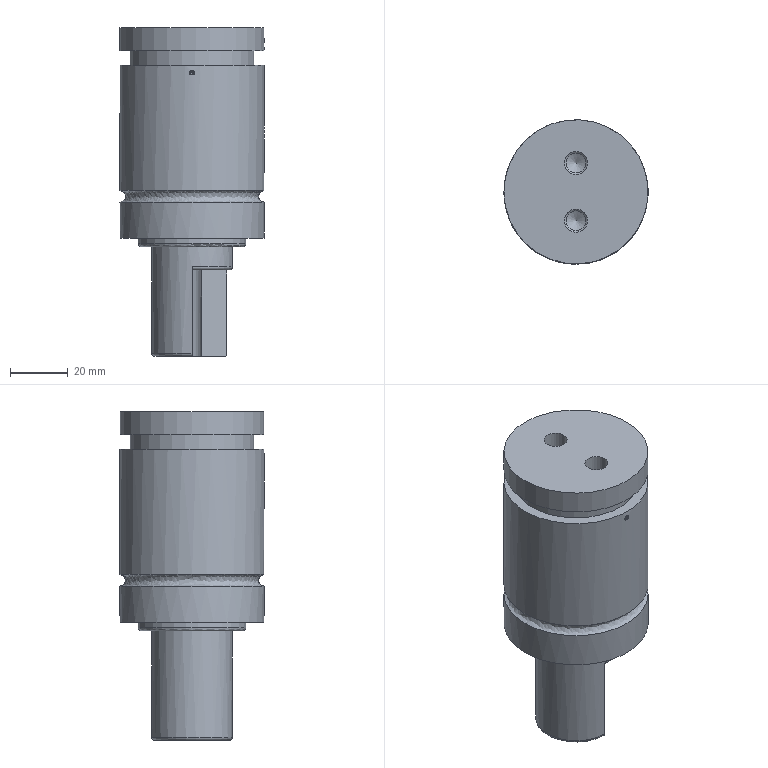Part | STEP file | GSV170-7_id1154_x_t | 1 solid | 183 faces | box 50 x 50 x 114 mm | volume 158224 mm3 | other 85 | plane 60 | cylinder 28 | cone 6 | torus 3 | spline 1 | commonest cylinder face diameters 50 x8 6.8 x3 8 x3 0.6 x1 0.859 x1 1.11 x1